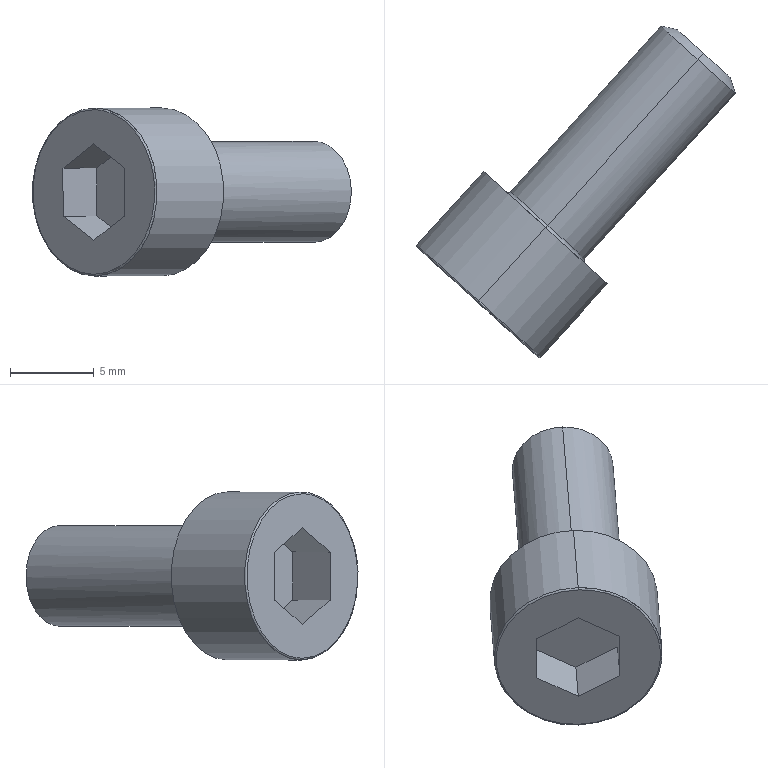Part | STEP file | PN_0025_Default<As Machined> | 1 solid | 20 faces | box 18.993 x 19.771 x 10.003 mm | volume 799.735 mm3 | plane 10 | torus 4 | cylinder 4 | cone 2 | commonest cylinder face diameters 6 x2 10 x2